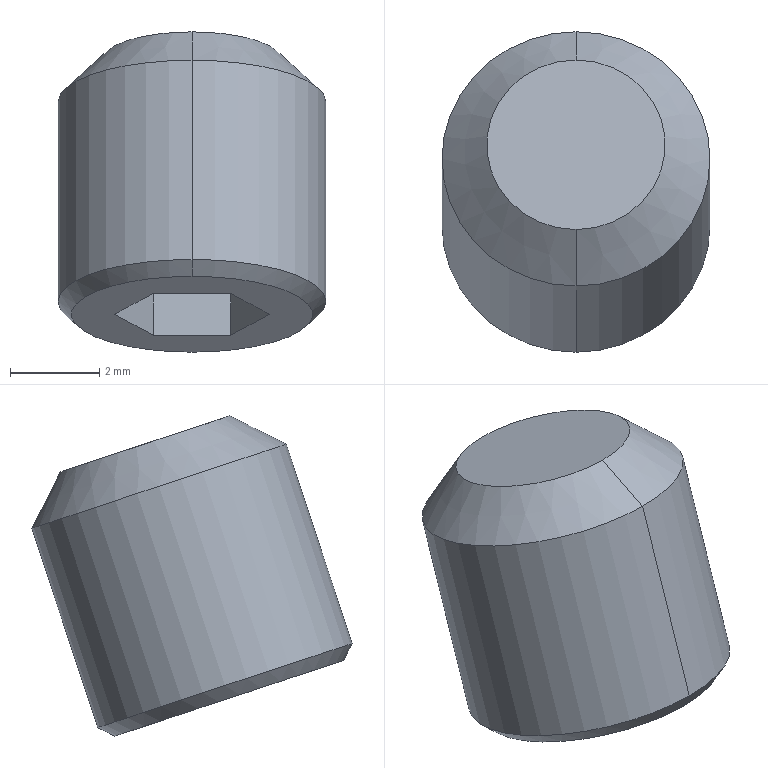Part | SolidWorks | features BaseBody 1 | 1 solid | 22 faces | box 6 x 7.172 x 7.172 mm | volume 142.819 mm3 | plane 14 | cone 6 | cylinder 2 | commonest cylinder face diameters 6 x2
STEP:
#1=CARTESIAN_POINT('',(-54.253,457.766,-361.285));
#2=VERTEX_POINT('',#1);
#3=CARTESIAN_POINT('',(-54.253,452.07,-359.401));
#4=VERTEX_POINT('',#3);
#5=CARTESIAN_POINT('',(-54.253,454.918,-360.343));
#6=DIRECTION('',(0.,-0.314,-0.9494));
#7=DIRECTION('',(0.,0.9494,-0.314));
#8=AXIS2_PLACEMENT_3D('',#5,#6,#7);
#9=CIRCLE('',#8,3.);
#10=EDGE_CURVE('',#2,#4,#9,.T.);
#11=ORIENTED_EDGE('',*,*,#10,.T.);
#12=CARTESIAN_POINT('',(-54.253,450.594,-363.863));
#13=VERTEX_POINT('',#12);
#14=CARTESIAN_POINT('',(-54.253,450.5,-364.148));
#15=DIRECTION('',(0.,-0.314,-0.9494));
#16=VECTOR('',#15,1000.);
#17=LINE('',#14,#16);
#18=EDGE_CURVE('',#4,#13,#17,.T.);
#19=ORIENTED_EDGE('',*,*,#18,.T.);
#20=CARTESIAN_POINT('',(-54.253,456.291,-365.747));
#21=VERTEX_POINT('',#20);
#22=CARTESIAN_POINT('',(-54.253,453.442,-364.805));
#23=DIRECTION('',(0.,0.314,0.9494));
#24=DIRECTION('',(0.,0.9494,-0.314));
#25=AXIS2_PLACEMENT_3D('',#22,#23,#24);
#26=CIRCLE('',#25,3.);
#27=EDGE_CURVE('',#13,#21,#26,.T.);
#28=ORIENTED_EDGE('',*,*,#27,.T.);
#29=CARTESIAN_POINT('',(-54.253,456.197,-366.032));
#30=DIRECTION('',(0.,-0.314,-0.9494));
#31=VECTOR('',#30,1000.);
#32=LINE('',#29,#31);
#33=EDGE_CURVE('',#2,#21,#32,.T.);
#34=ORIENTED_EDGE('',*,*,#33,.F.);
#35=EDGE_LOOP('',(#11,#19,#28,#34));
#36=FACE_OUTER_BOUND('',#35,.T.);
#37=CARTESIAN_POINT('',(-54.253,453.348,-365.09));
#38=DIRECTION('',(0.,-0.314,-0.9494));
#39=DIRECTION('',(0.,0.9494,-0.314));
#40=AXIS2_PLACEMENT_3D('',#37,#38,#39);
#41=CYLINDRICAL_SURFACE('',#40,3.);
#42=ADVANCED_FACE('',(#36),#41,.T.);
#43=CARTESIAN_POINT('',(-54.253,450.785,-364.242));
#44=VERTEX_POINT('',#43);
#45=CARTESIAN_POINT('',(-54.253,455.912,-365.937));
#46=VERTEX_POINT('',#45);
#47=CARTESIAN_POINT('',(-54.253,453.348,-365.09));
#48=DIRECTION('',(0.,0.314,0.9494));
#49=DIRECTION('',(0.,-0.9494,0.314));
#50=AXIS2_PLACEMENT_3D('',#47,#48,#49);
#51=CIRCLE('',#50,2.7);
#52=EDGE_CURVE('',#44,#46,#51,.T.);
#53=ORIENTED_EDGE('',*,*,#52,.T.);
#54=CARTESIAN_POINT('',(-54.253,456.291,-365.747));
#55=DIRECTION('',(0.,0.8934,0.4493));
#56=VECTOR('',#55,1000.);
#57=LINE('',#54,#56);
#58=EDGE_CURVE('',#46,#21,#57,.T.);
#59=ORIENTED_EDGE('',*,*,#58,.T.);
#60=ORIENTED_EDGE('',*,*,#27,.F.);
#61=CARTESIAN_POINT('',(-54.253,450.594,-363.863));
#62=DIRECTION('',(0.,-0.4493,0.8934));
#63=VECTOR('',#62,1000.);
#64=LINE('',#61,#63);
#65=EDGE_CURVE('',#44,#13,#64,.T.);
#66=ORIENTED_EDGE('',*,*,#65,.F.);
#67=EDGE_LOOP('',(#53,#59,#60,#66));
#68=FACE_OUTER_BOUND('',#67,.T.);
#69=CARTESIAN_POINT('',(-54.253,453.442,-364.805));
#70=DIRECTION('',(0.,0.314,0.9494));
#71=DIRECTION('',(0.,-0.9494,0.314));
#72=AXIS2_PLACEMENT_3D('',#69,#70,#71);
#73=CONICAL_SURFACE('',#72,3.,0.7854);
#74=ADVANCED_FACE('',(#68),#73,.T.);
#75=CARTESIAN_POINT('',(-54.253,457.131,-360.021));
#76=VERTEX_POINT('',#75);
#77=CARTESIAN_POINT('',(-54.253,453.333,-358.765));
#78=VERTEX_POINT('',#77);
#79=CARTESIAN_POINT('',(-54.253,455.232,-359.393));
#80=DIRECTION('',(0.,-0.314,-0.9494));
#81=DIRECTION('',(0.,0.9494,-0.314));
#82=AXIS2_PLACEMENT_3D('',#79,#80,#81);
#83=CIRCLE('',#82,2.);
#84=EDGE_CURVE('',#76,#78,#83,.T.);
#85=ORIENTED_EDGE('',*,*,#84,.T.);
#86=CARTESIAN_POINT('',(-54.253,452.07,-359.401));
#87=DIRECTION('',(0.,-0.8934,-0.4493));
#88=VECTOR('',#87,1000.);
#89=LINE('',#86,#88);
#90=EDGE_CURVE('',#78,#4,#89,.T.);
#91=ORIENTED_EDGE('',*,*,#90,.T.);
#92=ORIENTED_EDGE('',*,*,#10,.F.);
#93=CARTESIAN_POINT('',(-54.253,457.766,-361.285));
#94=DIRECTION('',(0.,0.4493,-0.8934));
#95=VECTOR('',#94,1000.);
#96=LINE('',#93,#95);
#97=EDGE_CURVE('',#76,#2,#96,.T.);
#98=ORIENTED_EDGE('',*,*,#97,.F.);
#99=EDGE_LOOP('',(#85,#91,#92,#98));
#100=FACE_OUTER_BOUND('',#99,.T.);
#101=CARTESIAN_POINT('',(-54.253,454.918,-360.343));
#102=DIRECTION('',(0.,-0.314,-0.9494));
#103=DIRECTION('',(0.,0.9494,-0.314));
#104=AXIS2_PLACEMENT_3D('',#101,#102,#103);
#105=CONICAL_SURFACE('',#104,3.,0.7854);
#106=ADVANCED_FACE('',(#100),#105,.T.);
#107=CARTESIAN_POINT('',(-54.253,454.248,-362.369));
#108=VERTEX_POINT('',#107);
#109=CARTESIAN_POINT('',(-54.253,455.4,-363.662));
#110=VERTEX_POINT('',#109);
#111=CARTESIAN_POINT('',(-54.253,455.4,-363.662));
#112=DIRECTION('',(0.,0.6652,-0.7466));
#113=VECTOR('',#112,1000.);
#114=LINE('',#111,#113);
#115=EDGE_CURVE('',#108,#110,#114,.T.);
#116=ORIENTED_EDGE('',*,*,#115,.F.);
#117=CARTESIAN_POINT('',(-54.253,452.552,-362.72));
#118=VERTEX_POINT('',#117);
#119=CARTESIAN_POINT('',(-54.253,452.552,-362.72));
#120=DIRECTION('',(0.,-0.9792,-0.2028));
#121=VECTOR('',#120,1000.);
#122=LINE('',#119,#121);
#123=EDGE_CURVE('',#108,#118,#122,.T.);
#124=ORIENTED_EDGE('',*,*,#123,.T.);
#125=CARTESIAN_POINT('',(-55.553,453.264,-362.955));
#126=VERTEX_POINT('',#125);
#127=CARTESIAN_POINT('',(-54.253,453.976,-363.191));
#128=DIRECTION('',(0.,-0.314,-0.9494));
#129=DIRECTION('',(0.,0.9494,-0.314));
#130=AXIS2_PLACEMENT_3D('',#127,#128,#129);
#131=CIRCLE('',#130,1.5);
#132=EDGE_CURVE('',#118,#126,#131,.T.);
#133=ORIENTED_EDGE('',*,*,#132,.T.);
#134=CARTESIAN_POINT('',(-55.553,454.688,-363.426));
#135=VERTEX_POINT('',#134);
#136=CARTESIAN_POINT('',(-54.253,453.976,-363.191));
#137=DIRECTION('',(0.,-0.314,-0.9494));
#138=DIRECTION('',(0.,0.9494,-0.314));
#139=AXIS2_PLACEMENT_3D('',#136,#137,#138);
#140=CIRCLE('',#139,1.5);
#141=EDGE_CURVE('',#126,#135,#140,.T.);
#142=ORIENTED_EDGE('',*,*,#141,.T.);
#143=CARTESIAN_POINT('',(-54.253,453.976,-363.191));
#144=DIRECTION('',(0.,-0.314,-0.9494));
#145=DIRECTION('',(0.,0.9494,-0.314));
#146=AXIS2_PLACEMENT_3D('',#143,#144,#145);
#147=CIRCLE('',#146,1.5);
#148=EDGE_CURVE('',#135,#110,#147,.T.);
#149=ORIENTED_EDGE('',*,*,#148,.T.);
#150=EDGE_LOOP('',(#116,#124,#133,#142,#149));
#151=FACE_OUTER_BOUND('',#150,.T.);
#152=CARTESIAN_POINT('',(-54.253,453.976,-363.191));
#153=DIRECTION('',(0.,-0.314,-0.9494));
#154=DIRECTION('',(0.,0.9494,-0.314));
#155=AXIS2_PLACEMENT_3D('',#152,#153,#154);
#156=CONICAL_SURFACE('',#155,1.5,1.047);
#157=ADVANCED_FACE('',(#151),#156,.F.);
#158=ORIENTED_EDGE('',*,*,#18,.F.);
#159=CARTESIAN_POINT('',(-54.253,454.918,-360.343));
#160=DIRECTION('',(0.,-0.314,-0.9494));
#161=DIRECTION('',(0.,0.9494,-0.314));
#162=AXIS2_PLACEMENT_3D('',#159,#160,#161);
#163=CIRCLE('',#162,3.);
#164=EDGE_CURVE('',#4,#2,#163,.T.);
#165=ORIENTED_EDGE('',*,*,#164,.T.);
#166=ORIENTED_EDGE('',*,*,#33,.T.);
#167=CARTESIAN_POINT('',(-54.253,453.442,-364.805));
#168=DIRECTION('',(0.,0.314,0.9494));
#169=DIRECTION('',(0.,0.9494,-0.314));
#170=AXIS2_PLACEMENT_3D('',#167,#168,#169);
#171=CIRCLE('',#170,3.);
#172=EDGE_CURVE('',#21,#13,#171,.T.);
#173=ORIENTED_EDGE('',*,*,#172,.T.);
#174=EDGE_LOOP('',(#158,#165,#166,#173));
#175=FACE_OUTER_BOUND('',#174,.T.);
#176=CARTESIAN_POINT('',(-54.253,453.348,-365.09));
#177=DIRECTION('',(0.,-0.314,-0.9494));
#178=DIRECTION('',(0.,0.9494,-0.314));
#179=AXIS2_PLACEMENT_3D('',#176,#177,#178);
#180=CYLINDRICAL_SURFACE('',#179,3.);
#181=ADVANCED_FACE('',(#175),#180,.T.);
#182=ORIENTED_EDGE('',*,*,#58,.F.);
#183=CARTESIAN_POINT('',(-54.253,453.348,-365.09));
#184=DIRECTION('',(0.,0.314,0.9494));
#185=DIRECTION('',(0.,-0.9494,0.314));
#186=AXIS2_PLACEMENT_3D('',#183,#184,#185);
#187=CIRCLE('',#186,2.7);
#188=EDGE_CURVE('',#46,#44,#187,.T.);
#189=ORIENTED_EDGE('',*,*,#188,.T.);
#190=ORIENTED_EDGE('',*,*,#65,.T.);
#191=ORIENTED_EDGE('',*,*,#172,.F.);
#192=EDGE_LOOP('',(#182,#189,#190,#191));
#193=FACE_OUTER_BOUND('',#192,.T.);
#194=CARTESIAN_POINT('',(-54.253,453.442,-364.805));
#195=DIRECTION('',(0.,0.314,0.9494));
#196=DIRECTION('',(0.,-0.9494,0.314));
#197=AXIS2_PLACEMENT_3D('',#194,#195,#196);
#198=CONICAL_SURFACE('',#197,3.,0.7854);
#199=ADVANCED_FACE('',(#193),#198,.T.);
#200=ORIENTED_EDGE('',*,*,#90,.F.);
#201=CARTESIAN_POINT('',(-54.253,455.232,-359.393));
#202=DIRECTION('',(0.,-0.314,-0.9494));
#203=DIRECTION('',(0.,0.9494,-0.314));
#204=AXIS2_PLACEMENT_3D('',#201,#202,#203);
#205=CIRCLE('',#204,2.);
#206=EDGE_CURVE('',#78,#76,#205,.T.);
#207=ORIENTED_EDGE('',*,*,#206,.T.);
#208=ORIENTED_EDGE('',*,*,#97,.T.);
#209=ORIENTED_EDGE('',*,*,#164,.F.);
#210=EDGE_LOOP('',(#200,#207,#208,#209));
#211=FACE_OUTER_BOUND('',#210,.T.);
#212=CARTESIAN_POINT('',(-54.253,454.918,-360.343));
#213=DIRECTION('',(0.,-0.314,-0.9494));
#214=DIRECTION('',(0.,0.9494,-0.314));
#215=AXIS2_PLACEMENT_3D('',#212,#213,#214);
#216=CONICAL_SURFACE('',#215,3.,0.7854);
#217=ADVANCED_FACE('',(#211),#216,.T.);
#218=CARTESIAN_POINT('',(-55.119,454.772,-365.561));
#219=VERTEX_POINT('',#218);
#220=CARTESIAN_POINT('',(-53.387,454.772,-365.561));
#221=VERTEX_POINT('',#220);
#222=CARTESIAN_POINT('',(-54.253,454.772,-365.561));
#223=DIRECTION('',(1.,0.,0.));
#224=VECTOR('',#223,1000.);
#225=LINE('',#222,#224);
#226=EDGE_CURVE('',#219,#221,#225,.T.);
#227=ORIENTED_EDGE('',*,*,#226,.F.);
#228=CARTESIAN_POINT('',(-55.986,453.348,-365.09));
#229=VERTEX_POINT('',#228);
#230=CARTESIAN_POINT('',(-55.986,453.348,-365.09));
#231=DIRECTION('',(0.5,0.8222,-0.2719));
#232=VECTOR('',#231,1000.);
#233=LINE('',#230,#232);
#234=EDGE_CURVE('',#229,#219,#233,.T.);
#235=ORIENTED_EDGE('',*,*,#234,.F.);
#236=CARTESIAN_POINT('',(-55.119,451.924,-364.619));
#237=VERTEX_POINT('',#236);
#238=CARTESIAN_POINT('',(-55.119,451.924,-364.619));
#239=DIRECTION('',(-0.5,0.8222,-0.2719));
#240=VECTOR('',#239,1000.);
#241=LINE('',#238,#240);
#242=EDGE_CURVE('',#237,#229,#241,.T.);
#243=ORIENTED_EDGE('',*,*,#242,.F.);
#244=CARTESIAN_POINT('',(-53.387,451.924,-364.619));
#245=VERTEX_POINT('',#244);
#246=CARTESIAN_POINT('',(-54.253,451.924,-364.619));
#247=DIRECTION('',(-1.,0.,0.));
#248=VECTOR('',#247,1000.);
#249=LINE('',#246,#248);
#250=EDGE_CURVE('',#245,#237,#249,.T.);
#251=ORIENTED_EDGE('',*,*,#250,.F.);
#252=CARTESIAN_POINT('',(-52.521,453.348,-365.09));
#253=VERTEX_POINT('',#252);
#254=CARTESIAN_POINT('',(-52.521,453.348,-365.09));
#255=DIRECTION('',(-0.5,-0.8222,0.2719));
#256=VECTOR('',#255,1000.);
#257=LINE('',#254,#256);
#258=EDGE_CURVE('',#253,#245,#257,.T.);
#259=ORIENTED_EDGE('',*,*,#258,.F.);
#260=CARTESIAN_POINT('',(-53.387,454.772,-365.561));
#261=DIRECTION('',(0.5,-0.8222,0.2719));
#262=VECTOR('',#261,1000.);
#263=LINE('',#260,#262);
#264=EDGE_CURVE('',#221,#253,#263,.T.);
#265=ORIENTED_EDGE('',*,*,#264,.F.);
#266=EDGE_LOOP('',(#227,#235,#243,#251,#259,#265));
#267=FACE_BOUND('',#266,.T.);
#268=ORIENTED_EDGE('',*,*,#52,.F.);
#269=ORIENTED_EDGE('',*,*,#188,.F.);
#270=EDGE_LOOP('',(#268,#269));
#271=FACE_OUTER_BOUND('',#270,.T.);
#272=CARTESIAN_POINT('',(-54.253,453.348,-365.09));
#273=DIRECTION('',(0.,0.314,0.9494));
#274=DIRECTION('',(0.,-0.9494,0.314));
#275=AXIS2_PLACEMENT_3D('',#272,#273,#274);
#276=PLANE('',#275);
#277=ADVANCED_FACE('',(#267,#271),#276,.F.);
#278=ORIENTED_EDGE('',*,*,#84,.F.);
#279=ORIENTED_EDGE('',*,*,#206,.F.);
#280=EDGE_LOOP('',(#278,#279));
#281=FACE_OUTER_BOUND('',#280,.T.);
#282=CARTESIAN_POINT('',(-54.253,455.232,-359.393));
#283=DIRECTION('',(0.,-0.314,-0.9494));
#284=DIRECTION('',(0.,0.9494,-0.314));
#285=AXIS2_PLACEMENT_3D('',#282,#283,#284);
#286=PLANE('',#285);
#287=ADVANCED_FACE('',(#281),#286,.F.);
#288=CARTESIAN_POINT('',(-53.387,455.4,-363.662));
#289=VERTEX_POINT('',#288);
#290=CARTESIAN_POINT('',(-53.387,455.4,-363.662));
#291=DIRECTION('',(0.,-0.314,-0.9494));
#292=VECTOR('',#291,1000.);
#293=LINE('',#290,#292);
#294=EDGE_CURVE('',#289,#221,#293,.T.);
#295=ORIENTED_EDGE('',*,*,#294,.T.);
#296=ORIENTED_EDGE('',*,*,#264,.T.);
#297=CARTESIAN_POINT('',(-52.521,453.976,-363.191));
#298=VERTEX_POINT('',#297);
#299=CARTESIAN_POINT('',(-52.521,453.348,-365.09));
#300=DIRECTION('',(0.,0.314,0.9494));
#301=VECTOR('',#300,1000.);
#302=LINE('',#299,#301);
#303=EDGE_CURVE('',#253,#298,#302,.T.);
#304=ORIENTED_EDGE('',*,*,#303,.T.);
#305=CARTESIAN_POINT('',(-52.954,454.688,-363.426));
#306=VERTEX_POINT('',#305);
#307=CARTESIAN_POINT('',(-52.521,453.976,-363.191));
#308=DIRECTION('',(-0.5,0.8222,-0.2719));
#309=VECTOR('',#308,1000.);
#310=LINE('',#307,#309);
#311=EDGE_CURVE('',#298,#306,#310,.T.);
#312=ORIENTED_EDGE('',*,*,#311,.T.);
#313=CARTESIAN_POINT('',(-52.954,454.688,-363.426));
#314=DIRECTION('',(-0.5,0.8222,-0.2719));
#315=VECTOR('',#314,1000.);
#316=LINE('',#313,#315);
#317=EDGE_CURVE('',#306,#289,#316,.T.);
#318=ORIENTED_EDGE('',*,*,#317,.T.);
#319=EDGE_LOOP('',(#295,#296,#304,#312,#318));
#320=FACE_OUTER_BOUND('',#319,.T.);
#321=CARTESIAN_POINT('',(-52.521,453.976,-363.191));
#322=DIRECTION('',(-0.866,-0.4747,0.157));
#323=DIRECTION('',(0.4807,-0.8769,0.));
#324=AXIS2_PLACEMENT_3D('',#321,#322,#323);
#325=PLANE('',#324);
#326=ADVANCED_FACE('',(#320),#325,.T.);
#327=CARTESIAN_POINT('',(-55.119,455.4,-363.662));
#328=VERTEX_POINT('',#327);
#329=CARTESIAN_POINT('',(-55.119,455.4,-363.662));
#330=DIRECTION('',(0.,-0.314,-0.9494));
#331=VECTOR('',#330,1000.);
#332=LINE('',#329,#331);
#333=EDGE_CURVE('',#328,#219,#332,.T.);
#334=ORIENTED_EDGE('',*,*,#333,.T.);
#335=ORIENTED_EDGE('',*,*,#226,.T.);
#336=ORIENTED_EDGE('',*,*,#294,.F.);
#337=CARTESIAN_POINT('',(-53.387,455.4,-363.662));
#338=DIRECTION('',(-1.,0.,0.));
#339=VECTOR('',#338,1000.);
#340=LINE('',#337,#339);
#341=EDGE_CURVE('',#289,#110,#340,.T.);
#342=ORIENTED_EDGE('',*,*,#341,.T.);
#343=CARTESIAN_POINT('',(-53.387,455.4,-363.662));
#344=DIRECTION('',(-1.,0.,0.));
#345=VECTOR('',#344,1000.);
#346=LINE('',#343,#345);
#347=EDGE_CURVE('',#110,#328,#346,.T.);
#348=ORIENTED_EDGE('',*,*,#347,.T.);
#349=EDGE_LOOP('',(#334,#335,#336,#342,#348));
#350=FACE_OUTER_BOUND('',#349,.T.);
#351=CARTESIAN_POINT('',(-53.387,455.4,-363.662));
#352=DIRECTION('',(0.,-0.9494,0.314));
#353=DIRECTION('',(0.,-0.314,-0.9494));
#354=AXIS2_PLACEMENT_3D('',#351,#352,#353);
#355=PLANE('',#354);
#356=ADVANCED_FACE('',(#350),#355,.T.);
#357=CARTESIAN_POINT('',(-55.986,453.976,-363.191));
#358=VERTEX_POINT('',#357);
#359=CARTESIAN_POINT('',(-55.986,453.976,-363.191));
#360=DIRECTION('',(0.,-0.314,-0.9494));
#361=VECTOR('',#360,1000.);
#362=LINE('',#359,#361);
#363=EDGE_CURVE('',#358,#229,#362,.T.);
#364=ORIENTED_EDGE('',*,*,#363,.T.);
#365=ORIENTED_EDGE('',*,*,#234,.T.);
#366=ORIENTED_EDGE('',*,*,#333,.F.);
#367=CARTESIAN_POINT('',(-55.119,455.4,-363.662));
#368=DIRECTION('',(-0.5,-0.8222,0.2719));
#369=VECTOR('',#368,1000.);
#370=LINE('',#367,#369);
#371=EDGE_CURVE('',#328,#135,#370,.T.);
#372=ORIENTED_EDGE('',*,*,#371,.T.);
#373=CARTESIAN_POINT('',(-55.553,454.688,-363.426));
#374=DIRECTION('',(-0.5,-0.8222,0.2719));
#375=VECTOR('',#374,1000.);
#376=LINE('',#373,#375);
#377=EDGE_CURVE('',#135,#358,#376,.T.);
#378=ORIENTED_EDGE('',*,*,#377,.T.);
#379=EDGE_LOOP('',(#364,#365,#366,#372,#378));
#380=FACE_OUTER_BOUND('',#379,.T.);
#381=CARTESIAN_POINT('',(-55.119,455.4,-363.662));
#382=DIRECTION('',(0.866,-0.4747,0.157));
#383=DIRECTION('',(0.4807,0.8769,0.));
#384=AXIS2_PLACEMENT_3D('',#381,#382,#383);
#385=PLANE('',#384);
#386=ADVANCED_FACE('',(#380),#385,.T.);
#387=CARTESIAN_POINT('',(-55.119,452.552,-362.72));
#388=VERTEX_POINT('',#387);
#389=CARTESIAN_POINT('',(-55.119,452.552,-362.72));
#390=DIRECTION('',(0.,-0.314,-0.9494));
#391=VECTOR('',#390,1000.);
#392=LINE('',#389,#391);
#393=EDGE_CURVE('',#388,#237,#392,.T.);
#394=ORIENTED_EDGE('',*,*,#393,.T.);
#395=ORIENTED_EDGE('',*,*,#242,.T.);
#396=ORIENTED_EDGE('',*,*,#363,.F.);
#397=CARTESIAN_POINT('',(-55.986,453.976,-363.191));
#398=DIRECTION('',(0.5,-0.8222,0.2719));
#399=VECTOR('',#398,1000.);
#400=LINE('',#397,#399);
#401=EDGE_CURVE('',#358,#126,#400,.T.);
#402=ORIENTED_EDGE('',*,*,#401,.T.);
#403=CARTESIAN_POINT('',(-55.553,453.264,-362.955));
#404=DIRECTION('',(0.5,-0.8222,0.2719));
#405=VECTOR('',#404,1000.);
#406=LINE('',#403,#405);
#407=EDGE_CURVE('',#126,#388,#406,.T.);
#408=ORIENTED_EDGE('',*,*,#407,.T.);
#409=EDGE_LOOP('',(#394,#395,#396,#402,#408));
#410=FACE_OUTER_BOUND('',#409,.T.);
#411=CARTESIAN_POINT('',(-55.986,453.976,-363.191));
#412=DIRECTION('',(0.866,0.4747,-0.157));
#413=DIRECTION('',(-0.4807,0.8769,0.));
#414=AXIS2_PLACEMENT_3D('',#411,#412,#413);
#415=PLANE('',#414);
#416=ADVANCED_FACE('',(#410),#415,.T.);
#417=CARTESIAN_POINT('',(-53.387,452.552,-362.72));
#418=VERTEX_POINT('',#417);
#419=CARTESIAN_POINT('',(-53.387,452.552,-362.72));
#420=DIRECTION('',(0.,-0.314,-0.9494));
#421=VECTOR('',#420,1000.);
#422=LINE('',#419,#421);
#423=EDGE_CURVE('',#418,#245,#422,.T.);
#424=ORIENTED_EDGE('',*,*,#423,.T.);
#425=ORIENTED_EDGE('',*,*,#250,.T.);
#426=ORIENTED_EDGE('',*,*,#393,.F.);
#427=CARTESIAN_POINT('',(-55.119,452.552,-362.72));
#428=DIRECTION('',(1.,0.,0.));
#429=VECTOR('',#428,1000.);
#430=LINE('',#427,#429);
#431=EDGE_CURVE('',#388,#118,#430,.T.);
#432=ORIENTED_EDGE('',*,*,#431,.T.);
#433=CARTESIAN_POINT('',(-55.119,452.552,-362.72));
#434=DIRECTION('',(1.,0.,0.));
#435=VECTOR('',#434,1000.);
#436=LINE('',#433,#435);
#437=EDGE_CURVE('',#118,#418,#436,.T.);
#438=ORIENTED_EDGE('',*,*,#437,.T.);
#439=EDGE_LOOP('',(#424,#425,#426,#432,#438));
#440=FACE_OUTER_BOUND('',#439,.T.);
#441=CARTESIAN_POINT('',(-55.119,452.552,-362.72));
#442=DIRECTION('',(0.,0.9494,-0.314));
#443=DIRECTION('',(0.,0.314,0.9494));
#444=AXIS2_PLACEMENT_3D('',#441,#442,#443);
#445=PLANE('',#444);
#446=ADVANCED_FACE('',(#440),#445,.T.);
#447=ORIENTED_EDGE('',*,*,#303,.F.);
#448=ORIENTED_EDGE('',*,*,#258,.T.);
#449=ORIENTED_EDGE('',*,*,#423,.F.);
#450=CARTESIAN_POINT('',(-52.954,453.264,-362.955));
#451=VERTEX_POINT('',#450);
#452=CARTESIAN_POINT('',(-53.387,452.552,-362.72));
#453=DIRECTION('',(0.5,0.8222,-0.2719));
#454=VECTOR('',#453,1000.);
#455=LINE('',#452,#454);
#456=EDGE_CURVE('',#418,#451,#455,.T.);
#457=ORIENTED_EDGE('',*,*,#456,.T.);
#458=CARTESIAN_POINT('',(-52.954,453.264,-362.955));
#459=DIRECTION('',(0.5,0.8222,-0.2719));
#460=VECTOR('',#459,1000.);
#461=LINE('',#458,#460);
#462=EDGE_CURVE('',#451,#298,#461,.T.);
#463=ORIENTED_EDGE('',*,*,#462,.T.);
#464=EDGE_LOOP('',(#447,#448,#449,#457,#463));
#465=FACE_OUTER_BOUND('',#464,.T.);
#466=CARTESIAN_POINT('',(-53.387,452.552,-362.72));
#467=DIRECTION('',(-0.866,0.4747,-0.157));
#468=DIRECTION('',(-0.4807,-0.8769,0.));
#469=AXIS2_PLACEMENT_3D('',#466,#467,#468);
#470=PLANE('',#469);
#471=ADVANCED_FACE('',(#465),#470,.T.);
#472=ORIENTED_EDGE('',*,*,#317,.F.);
#473=CARTESIAN_POINT('',(-54.253,453.976,-363.191));
#474=DIRECTION('',(0.,-0.314,-0.9494));
#475=DIRECTION('',(0.,0.9494,-0.314));
#476=AXIS2_PLACEMENT_3D('',#473,#474,#475);
#477=CIRCLE('',#476,1.5);
#478=EDGE_CURVE('',#110,#306,#477,.T.);
#479=ORIENTED_EDGE('',*,*,#478,.F.);
#480=ORIENTED_EDGE('',*,*,#341,.F.);
#481=EDGE_LOOP('',(#472,#479,#480));
#482=FACE_OUTER_BOUND('',#481,.T.);
#483=CARTESIAN_POINT('',(-54.253,453.976,-363.191));
#484=DIRECTION('',(0.,0.314,0.9494));
#485=DIRECTION('',(0.,-0.9494,0.314));
#486=AXIS2_PLACEMENT_3D('',#483,#484,#485);
#487=PLANE('',#486);
#488=ADVANCED_FACE('',(#482),#487,.F.);
#489=ORIENTED_EDGE('',*,*,#462,.F.);
#490=CARTESIAN_POINT('',(-54.253,453.976,-363.191));
#491=DIRECTION('',(0.,-0.314,-0.9494));
#492=DIRECTION('',(0.,0.9494,-0.314));
#493=AXIS2_PLACEMENT_3D('',#490,#491,#492);
#494=CIRCLE('',#493,1.5);
#495=EDGE_CURVE('',#306,#451,#494,.T.);
#496=ORIENTED_EDGE('',*,*,#495,.F.);
#497=ORIENTED_EDGE('',*,*,#311,.F.);
#498=EDGE_LOOP('',(#489,#496,#497));
#499=FACE_OUTER_BOUND('',#498,.T.);
#500=CARTESIAN_POINT('',(-54.253,453.976,-363.191));
#501=DIRECTION('',(0.,0.314,0.9494));
#502=DIRECTION('',(0.,-0.9494,0.314));
#503=AXIS2_PLACEMENT_3D('',#500,#501,#502);
#504=PLANE('',#503);
#505=ADVANCED_FACE('',(#499),#504,.F.);
#506=ORIENTED_EDGE('',*,*,#347,.F.);
#507=ORIENTED_EDGE('',*,*,#148,.F.);
#508=ORIENTED_EDGE('',*,*,#371,.F.);
#509=EDGE_LOOP('',(#506,#507,#508));
#510=FACE_OUTER_BOUND('',#509,.T.);
#511=CARTESIAN_POINT('',(-54.253,453.976,-363.191));
#512=DIRECTION('',(0.,0.314,0.9494));
#513=DIRECTION('',(0.,-0.9494,0.314));
#514=AXIS2_PLACEMENT_3D('',#511,#512,#513);
#515=PLANE('',#514);
#516=ADVANCED_FACE('',(#510),#515,.F.);
#517=ORIENTED_EDGE('',*,*,#377,.F.);
#518=ORIENTED_EDGE('',*,*,#141,.F.);
#519=ORIENTED_EDGE('',*,*,#401,.F.);
#520=EDGE_LOOP('',(#517,#518,#519));
#521=FACE_OUTER_BOUND('',#520,.T.);
#522=CARTESIAN_POINT('',(-54.253,453.976,-363.191));
#523=DIRECTION('',(0.,0.314,0.9494));
#524=DIRECTION('',(0.,-0.9494,0.314));
#525=AXIS2_PLACEMENT_3D('',#522,#523,#524);
#526=PLANE('',#525);
#527=ADVANCED_FACE('',(#521),#526,.F.);
#528=ORIENTED_EDGE('',*,*,#407,.F.);
#529=ORIENTED_EDGE('',*,*,#132,.F.);
#530=ORIENTED_EDGE('',*,*,#431,.F.);
#531=EDGE_LOOP('',(#528,#529,#530));
#532=FACE_OUTER_BOUND('',#531,.T.);
#533=CARTESIAN_POINT('',(-54.253,453.976,-363.191));
#534=DIRECTION('',(0.,0.314,0.9494));
#535=DIRECTION('',(0.,-0.9494,0.314));
#536=AXIS2_PLACEMENT_3D('',#533,#534,#535);
#537=PLANE('',#536);
#538=ADVANCED_FACE('',(#532),#537,.F.);
#539=ORIENTED_EDGE('',*,*,#437,.F.);
#540=CARTESIAN_POINT('',(-54.253,453.976,-363.191));
#541=DIRECTION('',(0.,-0.314,-0.9494));
#542=DIRECTION('',(0.,0.9494,-0.314));
#543=AXIS2_PLACEMENT_3D('',#540,#541,#542);
#544=CIRCLE('',#543,1.5);
#545=EDGE_CURVE('',#451,#118,#544,.T.);
#546=ORIENTED_EDGE('',*,*,#545,.F.);
#547=ORIENTED_EDGE('',*,*,#456,.F.);
#548=EDGE_LOOP('',(#539,#546,#547));
#549=FACE_OUTER_BOUND('',#548,.T.);
#550=CARTESIAN_POINT('',(-54.253,453.976,-363.191));
#551=DIRECTION('',(0.,0.314,0.9494));
#552=DIRECTION('',(0.,-0.9494,0.314));
#553=AXIS2_PLACEMENT_3D('',#550,#551,#552);
#554=PLANE('',#553);
#555=ADVANCED_FACE('',(#549),#554,.F.);
#556=ORIENTED_EDGE('',*,*,#123,.F.);
#557=ORIENTED_EDGE('',*,*,#115,.T.);
#558=ORIENTED_EDGE('',*,*,#478,.T.);
#559=ORIENTED_EDGE('',*,*,#495,.T.);
#560=ORIENTED_EDGE('',*,*,#545,.T.);
#561=EDGE_LOOP('',(#556,#557,#558,#559,#560));
#562=FACE_OUTER_BOUND('',#561,.T.);
#563=CARTESIAN_POINT('',(-54.253,453.976,-363.191));
#564=DIRECTION('',(0.,-0.314,-0.9494));
#565=DIRECTION('',(0.,0.9494,-0.314));
#566=AXIS2_PLACEMENT_3D('',#563,#564,#565);
#567=CONICAL_SURFACE('',#566,1.5,1.047);
#568=ADVANCED_FACE('',(#562),#567,.F.);
#569=CLOSED_SHELL('',(#42,#74,#106,#157,#181,#199,#217,#277,#287,#326,#356,#386,#416,#446,#471,#488,#505,#516,#527,#538,#555,#568));
#570=MANIFOLD_SOLID_BREP('',#569);
#571=CARTESIAN_POINT('',(0.,0.,0.));
#572=DIRECTION('',(0.,0.,1.));
#573=DIRECTION('',(1.,0.,0.));
#574=AXIS2_PLACEMENT_3D('',#571,#572,#573);
#575=(LENGTH_UNIT()NAMED_UNIT(*)SI_UNIT(.MILLI.,.METRE.));
#576=UNCERTAINTY_MEASURE_WITH_UNIT(LENGTH_MEASURE(0.00001),#575,'','');
#577=(NAMED_UNIT(*)PLANE_ANGLE_UNIT()SI_UNIT($,.RADIAN.));
#578=(NAMED_UNIT(*)SI_UNIT($,.STERADIAN.)SOLID_ANGLE_UNIT());
#579=(GEOMETRIC_REPRESENTATION_CONTEXT(3)GLOBAL_UNCERTAINTY_ASSIGNED_CONTEXT((#576))GLOBAL_UNIT_ASSIGNED_CONTEXT((#575,#577,#578))REPRESENTATION_CONTEXT('',''));
#580=ADVANCED_BREP_SHAPE_REPRESENTATION('',(#570,#574),#579);